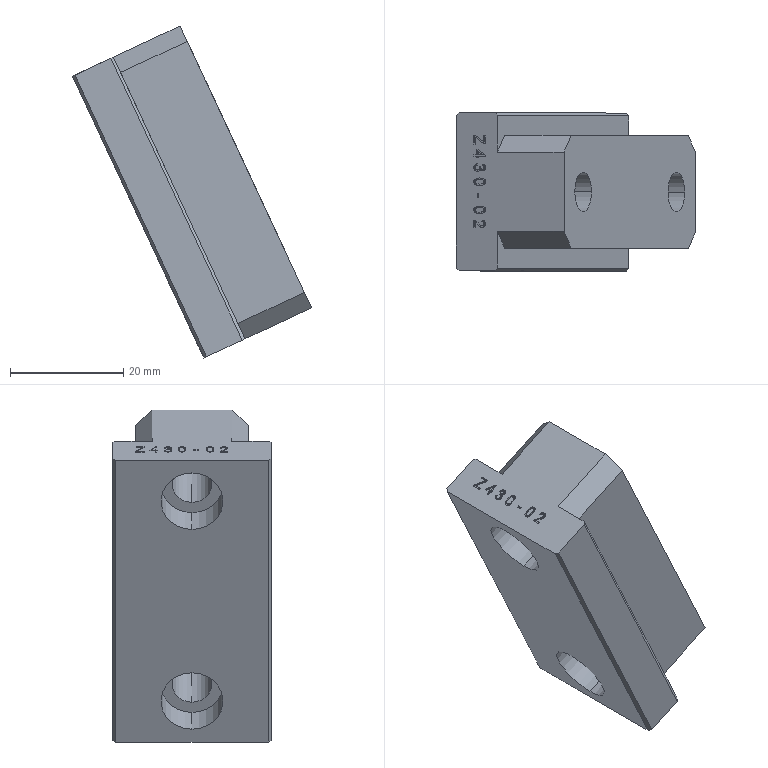Part | Creo | 1 solid | 160 faces | box 42.276 x 28 x 58.722 mm | volume 23949 mm3 | other 93 | plane 57 | cylinder 10 | commonest cylinder face diameters 7 x4 11 x4 1.927 x1 30.388 x1